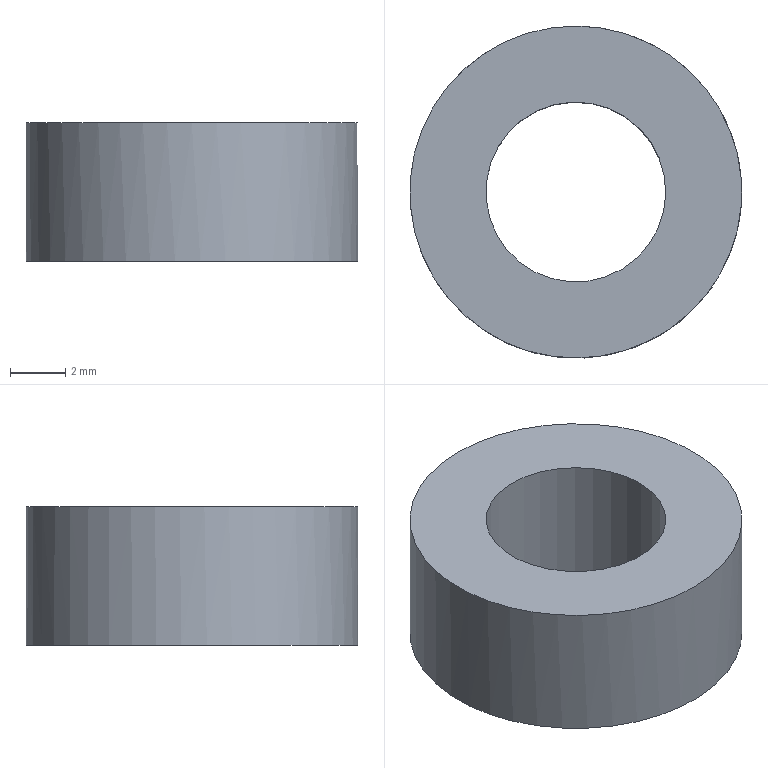Part | STEP file | lll_id58_x_t | 1 solid | 4 faces | box 12 x 12 x 5 mm | volume 399.571 mm3 | plane 2 | cylinder 2 | commonest cylinder face diameters 6.5 x1 12 x1
STEP:
#1=CARTESIAN_POINT('',(776.917,31.045,-8.));
#2=VERTEX_POINT('',#1);
#3=CARTESIAN_POINT('',(779.732,29.42,-8.));
#4=DIRECTION('',(0.,0.,-1.));
#5=DIRECTION('',(-0.866,0.5,0.));
#6=AXIS2_PLACEMENT_3D('',#3,#4,#5);
#7=CIRCLE('',#6,3.25);
#8=EDGE_CURVE('',#2,#2,#7,.T.);
#9=ORIENTED_EDGE('',*,*,#8,.T.);
#10=EDGE_LOOP('',(#9));
#11=FACE_BOUND('',#10,.T.);
#12=CARTESIAN_POINT('',(784.928,26.42,-8.));
#13=VERTEX_POINT('',#12);
#14=CARTESIAN_POINT('',(779.732,29.42,-8.));
#15=DIRECTION('',(0.,0.,-1.));
#16=DIRECTION('',(0.866,-0.5,0.));
#17=AXIS2_PLACEMENT_3D('',#14,#15,#16);
#18=CIRCLE('',#17,6.);
#19=EDGE_CURVE('',#13,#13,#18,.T.);
#20=ORIENTED_EDGE('',*,*,#19,.F.);
#21=EDGE_LOOP('',(#20));
#22=FACE_BOUND('',#21,.T.);
#23=CARTESIAN_POINT('',(779.732,29.42,-8.));
#24=DIRECTION('',(0.,0.,1.));
#25=DIRECTION('',(-1.,0.,0.));
#26=AXIS2_PLACEMENT_3D('',#23,#24,#25);
#27=PLANE('',#26);
#28=ADVANCED_FACE('',(#11,#22),#27,.T.);
#29=CARTESIAN_POINT('',(776.917,31.045,-13.));
#30=VERTEX_POINT('',#29);
#31=CARTESIAN_POINT('',(779.732,29.42,-13.));
#32=DIRECTION('',(0.,0.,-1.));
#33=DIRECTION('',(-0.866,0.5,0.));
#34=AXIS2_PLACEMENT_3D('',#31,#32,#33);
#35=CIRCLE('',#34,3.25);
#36=EDGE_CURVE('',#30,#30,#35,.T.);
#37=ORIENTED_EDGE('',*,*,#36,.F.);
#38=EDGE_LOOP('',(#37));
#39=FACE_BOUND('',#38,.T.);
#40=CARTESIAN_POINT('',(774.536,32.42,-13.));
#41=VERTEX_POINT('',#40);
#42=CARTESIAN_POINT('',(779.732,29.42,-13.));
#43=DIRECTION('',(0.,0.,1.));
#44=DIRECTION('',(-0.866,0.5,0.));
#45=AXIS2_PLACEMENT_3D('',#42,#43,#44);
#46=CIRCLE('',#45,6.);
#47=EDGE_CURVE('',#41,#41,#46,.T.);
#48=ORIENTED_EDGE('',*,*,#47,.F.);
#49=EDGE_LOOP('',(#48));
#50=FACE_BOUND('',#49,.T.);
#51=CARTESIAN_POINT('',(779.732,29.42,-13.));
#52=DIRECTION('',(0.,0.,-1.));
#53=DIRECTION('',(1.,0.,0.));
#54=AXIS2_PLACEMENT_3D('',#51,#52,#53);
#55=PLANE('',#54);
#56=ADVANCED_FACE('',(#39,#50),#55,.T.);
#57=ORIENTED_EDGE('',*,*,#19,.T.);
#58=EDGE_LOOP('',(#57));
#59=FACE_BOUND('',#58,.T.);
#60=ORIENTED_EDGE('',*,*,#47,.T.);
#61=EDGE_LOOP('',(#60));
#62=FACE_BOUND('',#61,.T.);
#63=CARTESIAN_POINT('',(779.732,29.42,-13.));
#64=DIRECTION('',(0.,0.,1.));
#65=DIRECTION('',(-1.,0.,0.));
#66=AXIS2_PLACEMENT_3D('',#63,#64,#65);
#67=CYLINDRICAL_SURFACE('',#66,6.);
#68=ADVANCED_FACE('',(#59,#62),#67,.T.);
#69=ORIENTED_EDGE('',*,*,#36,.T.);
#70=EDGE_LOOP('',(#69));
#71=FACE_BOUND('',#70,.T.);
#72=ORIENTED_EDGE('',*,*,#8,.F.);
#73=EDGE_LOOP('',(#72));
#74=FACE_BOUND('',#73,.T.);
#75=CARTESIAN_POINT('',(779.732,29.42,-8.));
#76=DIRECTION('',(0.,0.,-1.));
#77=DIRECTION('',(-0.866,0.5,0.));
#78=AXIS2_PLACEMENT_3D('',#75,#76,#77);
#79=CYLINDRICAL_SURFACE('',#78,3.25);
#80=ADVANCED_FACE('',(#71,#74),#79,.F.);
#81=CLOSED_SHELL('',(#28,#56,#68,#80));
#82=MANIFOLD_SOLID_BREP('',#81);
#83=(LENGTH_UNIT()NAMED_UNIT(*)SI_UNIT(.MILLI.,.METRE.));
#84=UNCERTAINTY_MEASURE_WITH_UNIT(LENGTH_MEASURE(0.00002),#83,'','');
#85=(NAMED_UNIT(*)PLANE_ANGLE_UNIT()SI_UNIT($,.RADIAN.));
#86=PLANE_ANGLE_MEASURE_WITH_UNIT(PLANE_ANGLE_MEASURE(0.01745),#85);
#87=DIMENSIONAL_EXPONENTS(0.,0.,0.,0.,0.,0.,0.);
#88=(CONVERSION_BASED_UNIT('DEGREE',#86)NAMED_UNIT(#87)PLANE_ANGLE_UNIT());
#89=(NAMED_UNIT(*)SI_UNIT($,.STERADIAN.)SOLID_ANGLE_UNIT());
#90=(GEOMETRIC_REPRESENTATION_CONTEXT(3)GLOBAL_UNCERTAINTY_ASSIGNED_CONTEXT((#84))GLOBAL_UNIT_ASSIGNED_CONTEXT((#83,#88,#89))REPRESENTATION_CONTEXT('',''));
#91=ADVANCED_BREP_SHAPE_REPRESENTATION('',(#82),#90);